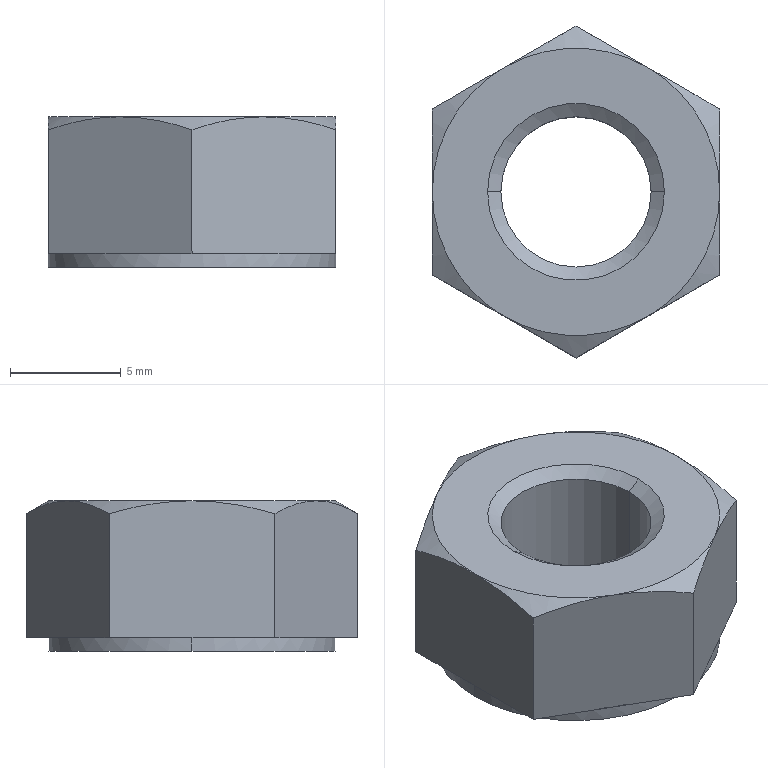Part | STEP file | hex nut style 1 gradeab_iso_ISO - 4032 - M8 - W - N | 1 solid | 30 faces | box 13 x 15.011 x 6.8 mm | volume 731.665 mm3 | plane 14 | cone 10 | cylinder 6 | commonest cylinder face diameters 6.8 x2 8 x2 13 x2
STEP:
#1=CARTESIAN_POINT('',(-4.,0.,-6.8));
#2=VERTEX_POINT('',#1);
#3=CARTESIAN_POINT('',(4.,0.,-6.8));
#4=VERTEX_POINT('',#3);
#5=CARTESIAN_POINT('',(0.,0.,-6.8));
#6=DIRECTION('',(0.,0.,1.));
#7=DIRECTION('',(-1.,0.,0.));
#8=AXIS2_PLACEMENT_3D('',#5,#6,#7);
#9=CIRCLE('',#8,4.);
#10=EDGE_CURVE('',#2,#4,#9,.T.);
#11=ORIENTED_EDGE('',*,*,#10,.F.);
#12=CARTESIAN_POINT('',(-4.,0.,-6.775));
#13=VERTEX_POINT('',#12);
#14=CARTESIAN_POINT('',(-4.,0.,-25.038));
#15=DIRECTION('',(0.,0.,1.));
#16=VECTOR('',#15,1000.);
#17=LINE('',#14,#16);
#18=EDGE_CURVE('',#2,#13,#17,.T.);
#19=ORIENTED_EDGE('',*,*,#18,.T.);
#20=CARTESIAN_POINT('',(4.,0.,-6.775));
#21=VERTEX_POINT('',#20);
#22=CARTESIAN_POINT('',(0.,0.,-6.775));
#23=DIRECTION('',(0.,0.,1.));
#24=DIRECTION('',(1.,0.,0.));
#25=AXIS2_PLACEMENT_3D('',#22,#23,#24);
#26=CIRCLE('',#25,4.);
#27=EDGE_CURVE('',#13,#21,#26,.T.);
#28=ORIENTED_EDGE('',*,*,#27,.T.);
#29=CARTESIAN_POINT('',(4.,0.,-25.038));
#30=DIRECTION('',(0.,0.,1.));
#31=VECTOR('',#30,1000.);
#32=LINE('',#29,#31);
#33=EDGE_CURVE('',#4,#21,#32,.T.);
#34=ORIENTED_EDGE('',*,*,#33,.F.);
#35=EDGE_LOOP('',(#11,#19,#28,#34));
#36=FACE_OUTER_BOUND('',#35,.T.);
#37=CARTESIAN_POINT('',(0.,0.,-25.038));
#38=DIRECTION('',(0.,0.,1.));
#39=DIRECTION('',(1.,0.,0.));
#40=AXIS2_PLACEMENT_3D('',#37,#38,#39);
#41=CYLINDRICAL_SURFACE('',#40,4.);
#42=ADVANCED_FACE('',(#36),#41,.F.);
#43=CARTESIAN_POINT('',(-3.4,0.,-6.354));
#44=VERTEX_POINT('',#43);
#45=CARTESIAN_POINT('',(3.4,0.,-6.354));
#46=VERTEX_POINT('',#45);
#47=CARTESIAN_POINT('',(0.,0.,-6.354));
#48=DIRECTION('',(0.,0.,1.));
#49=DIRECTION('',(-1.,0.,0.));
#50=AXIS2_PLACEMENT_3D('',#47,#48,#49);
#51=CIRCLE('',#50,3.4);
#52=EDGE_CURVE('',#44,#46,#51,.T.);
#53=ORIENTED_EDGE('',*,*,#52,.T.);
#54=CARTESIAN_POINT('',(4.,0.,-6.775));
#55=DIRECTION('',(0.8192,0.,-0.5736));
#56=VECTOR('',#55,1000.);
#57=LINE('',#54,#56);
#58=EDGE_CURVE('',#46,#21,#57,.T.);
#59=ORIENTED_EDGE('',*,*,#58,.T.);
#60=ORIENTED_EDGE('',*,*,#27,.F.);
#61=CARTESIAN_POINT('',(-4.,0.,-6.775));
#62=DIRECTION('',(-0.8192,0.,-0.5736));
#63=VECTOR('',#62,1000.);
#64=LINE('',#61,#63);
#65=EDGE_CURVE('',#44,#13,#64,.T.);
#66=ORIENTED_EDGE('',*,*,#65,.F.);
#67=EDGE_LOOP('',(#53,#59,#60,#66));
#68=FACE_OUTER_BOUND('',#67,.T.);
#69=CARTESIAN_POINT('',(0.,0.,-6.775));
#70=DIRECTION('',(0.,0.,-1.));
#71=DIRECTION('',(-1.,0.,0.));
#72=AXIS2_PLACEMENT_3D('',#69,#70,#71);
#73=CONICAL_SURFACE('',#72,4.,0.9599);
#74=ADVANCED_FACE('',(#68),#73,.F.);
#75=CARTESIAN_POINT('',(3.4,0.,-0.4201));
#76=VERTEX_POINT('',#75);
#77=CARTESIAN_POINT('',(-3.4,0.,-0.4201));
#78=VERTEX_POINT('',#77);
#79=CARTESIAN_POINT('',(0.,0.,-0.4201));
#80=DIRECTION('',(0.,0.,-1.));
#81=DIRECTION('',(1.,0.,0.));
#82=AXIS2_PLACEMENT_3D('',#79,#80,#81);
#83=CIRCLE('',#82,3.4);
#84=EDGE_CURVE('',#76,#78,#83,.T.);
#85=ORIENTED_EDGE('',*,*,#84,.T.);
#86=CARTESIAN_POINT('',(-4.,0.,0.));
#87=VERTEX_POINT('',#86);
#88=CARTESIAN_POINT('',(-3.34,0.,-0.4621));
#89=DIRECTION('',(-0.8192,0.,0.5736));
#90=VECTOR('',#89,1000.);
#91=LINE('',#88,#90);
#92=EDGE_CURVE('',#78,#87,#91,.T.);
#93=ORIENTED_EDGE('',*,*,#92,.T.);
#94=CARTESIAN_POINT('',(4.,0.,0.));
#95=VERTEX_POINT('',#94);
#96=CARTESIAN_POINT('',(0.,0.,0.));
#97=DIRECTION('',(0.,0.,1.));
#98=DIRECTION('',(1.,0.,0.));
#99=AXIS2_PLACEMENT_3D('',#96,#97,#98);
#100=CIRCLE('',#99,4.);
#101=EDGE_CURVE('',#87,#95,#100,.T.);
#102=ORIENTED_EDGE('',*,*,#101,.T.);
#103=CARTESIAN_POINT('',(3.34,0.,-0.4621));
#104=DIRECTION('',(0.8192,0.,0.5736));
#105=VECTOR('',#104,1000.);
#106=LINE('',#103,#105);
#107=EDGE_CURVE('',#76,#95,#106,.T.);
#108=ORIENTED_EDGE('',*,*,#107,.F.);
#109=EDGE_LOOP('',(#85,#93,#102,#108));
#110=FACE_OUTER_BOUND('',#109,.T.);
#111=CARTESIAN_POINT('',(0.,0.,-0.4621));
#112=DIRECTION('',(0.,0.,1.));
#113=DIRECTION('',(1.,0.,0.));
#114=AXIS2_PLACEMENT_3D('',#111,#112,#113);
#115=CONICAL_SURFACE('',#114,3.34,0.9599);
#116=ADVANCED_FACE('',(#110),#115,.F.);
#117=CARTESIAN_POINT('',(6.5,0.,-6.8));
#118=VERTEX_POINT('',#117);
#119=CARTESIAN_POINT('',(-6.5,0.,-6.8));
#120=VERTEX_POINT('',#119);
#121=CARTESIAN_POINT('',(0.,0.,-6.8));
#122=DIRECTION('',(0.,0.,1.));
#123=DIRECTION('',(-1.,0.,0.));
#124=AXIS2_PLACEMENT_3D('',#121,#122,#123);
#125=CIRCLE('',#124,6.5);
#126=EDGE_CURVE('',#118,#120,#125,.T.);
#127=ORIENTED_EDGE('',*,*,#126,.T.);
#128=CARTESIAN_POINT('',(-6.5,0.,-6.2));
#129=VERTEX_POINT('',#128);
#130=CARTESIAN_POINT('',(-6.5,0.,0.));
#131=DIRECTION('',(0.,0.,1.));
#132=VECTOR('',#131,1000.);
#133=LINE('',#130,#132);
#134=EDGE_CURVE('',#120,#129,#133,.T.);
#135=ORIENTED_EDGE('',*,*,#134,.T.);
#136=CARTESIAN_POINT('',(-3.25,5.629,-6.2));
#137=VERTEX_POINT('',#136);
#138=CARTESIAN_POINT('',(0.,0.,-6.2));
#139=DIRECTION('',(0.,0.,1.));
#140=DIRECTION('',(1.,0.,0.));
#141=AXIS2_PLACEMENT_3D('',#138,#139,#140);
#142=CIRCLE('',#141,6.5);
#143=EDGE_CURVE('',#137,#129,#142,.T.);
#144=ORIENTED_EDGE('',*,*,#143,.F.);
#145=CARTESIAN_POINT('',(3.25,5.629,-6.2));
#146=VERTEX_POINT('',#145);
#147=CARTESIAN_POINT('',(0.,0.,-6.2));
#148=DIRECTION('',(0.,0.,1.));
#149=DIRECTION('',(1.,0.,0.));
#150=AXIS2_PLACEMENT_3D('',#147,#148,#149);
#151=CIRCLE('',#150,6.5);
#152=EDGE_CURVE('',#146,#137,#151,.T.);
#153=ORIENTED_EDGE('',*,*,#152,.F.);
#154=CARTESIAN_POINT('',(6.5,0.,-6.2));
#155=VERTEX_POINT('',#154);
#156=CARTESIAN_POINT('',(0.,0.,-6.2));
#157=DIRECTION('',(0.,0.,1.));
#158=DIRECTION('',(1.,0.,0.));
#159=AXIS2_PLACEMENT_3D('',#156,#157,#158);
#160=CIRCLE('',#159,6.5);
#161=EDGE_CURVE('',#155,#146,#160,.T.);
#162=ORIENTED_EDGE('',*,*,#161,.F.);
#163=CARTESIAN_POINT('',(6.5,0.,0.));
#164=DIRECTION('',(0.,0.,1.));
#165=VECTOR('',#164,1000.);
#166=LINE('',#163,#165);
#167=EDGE_CURVE('',#118,#155,#166,.T.);
#168=ORIENTED_EDGE('',*,*,#167,.F.);
#169=EDGE_LOOP('',(#127,#135,#144,#153,#162,#168));
#170=FACE_OUTER_BOUND('',#169,.T.);
#171=CARTESIAN_POINT('',(0.,0.,0.));
#172=DIRECTION('',(0.,0.,1.));
#173=DIRECTION('',(1.,0.,0.));
#174=AXIS2_PLACEMENT_3D('',#171,#172,#173);
#175=CYLINDRICAL_SURFACE('',#174,6.5);
#176=ADVANCED_FACE('',(#170),#175,.T.);
#177=ORIENTED_EDGE('',*,*,#52,.F.);
#178=CARTESIAN_POINT('',(-3.4,0.,-6.8));
#179=DIRECTION('',(0.,0.,1.));
#180=VECTOR('',#179,1000.);
#181=LINE('',#178,#180);
#182=EDGE_CURVE('',#44,#78,#181,.T.);
#183=ORIENTED_EDGE('',*,*,#182,.T.);
#184=ORIENTED_EDGE('',*,*,#84,.F.);
#185=CARTESIAN_POINT('',(3.4,0.,-6.8));
#186=DIRECTION('',(0.,0.,1.));
#187=VECTOR('',#186,1000.);
#188=LINE('',#185,#187);
#189=EDGE_CURVE('',#46,#76,#188,.T.);
#190=ORIENTED_EDGE('',*,*,#189,.F.);
#191=EDGE_LOOP('',(#177,#183,#184,#190));
#192=FACE_OUTER_BOUND('',#191,.T.);
#193=CARTESIAN_POINT('',(0.,0.,-6.8));
#194=DIRECTION('',(0.,0.,1.));
#195=DIRECTION('',(1.,0.,0.));
#196=AXIS2_PLACEMENT_3D('',#193,#194,#195);
#197=CYLINDRICAL_SURFACE('',#196,3.4);
#198=ADVANCED_FACE('',(#192),#197,.F.);
#199=ORIENTED_EDGE('',*,*,#182,.F.);
#200=CARTESIAN_POINT('',(0.,0.,-6.354));
#201=DIRECTION('',(0.,0.,1.));
#202=DIRECTION('',(-1.,0.,0.));
#203=AXIS2_PLACEMENT_3D('',#200,#201,#202);
#204=CIRCLE('',#203,3.4);
#205=EDGE_CURVE('',#46,#44,#204,.T.);
#206=ORIENTED_EDGE('',*,*,#205,.F.);
#207=ORIENTED_EDGE('',*,*,#189,.T.);
#208=CARTESIAN_POINT('',(0.,0.,-0.4201));
#209=DIRECTION('',(0.,0.,-1.));
#210=DIRECTION('',(1.,0.,0.));
#211=AXIS2_PLACEMENT_3D('',#208,#209,#210);
#212=CIRCLE('',#211,3.4);
#213=EDGE_CURVE('',#78,#76,#212,.T.);
#214=ORIENTED_EDGE('',*,*,#213,.F.);
#215=EDGE_LOOP('',(#199,#206,#207,#214));
#216=FACE_OUTER_BOUND('',#215,.T.);
#217=CARTESIAN_POINT('',(0.,0.,-6.8));
#218=DIRECTION('',(0.,0.,1.));
#219=DIRECTION('',(1.,0.,0.));
#220=AXIS2_PLACEMENT_3D('',#217,#218,#219);
#221=CYLINDRICAL_SURFACE('',#220,3.4);
#222=ADVANCED_FACE('',(#216),#221,.F.);
#223=CARTESIAN_POINT('',(-6.5,3.753,-6.2));
#224=VERTEX_POINT('',#223);
#225=CARTESIAN_POINT('',(-6.5,3.753,-0.5806));
#226=VERTEX_POINT('',#225);
#227=CARTESIAN_POINT('',(-6.5,3.753,-6.8));
#228=DIRECTION('',(0.,0.,1.));
#229=VECTOR('',#228,1000.);
#230=LINE('',#227,#229);
#231=EDGE_CURVE('',#224,#226,#230,.T.);
#232=ORIENTED_EDGE('',*,*,#231,.T.);
#233=CARTESIAN_POINT('',(-3.25,5.629,0.));
#234=VERTEX_POINT('',#233);
#235=CARTESIAN_POINT('',(-6.5,3.753,-0.5806));
#236=CARTESIAN_POINT('',(-5.968,4.06,-0.4033));
#237=CARTESIAN_POINT('',(-5.433,4.369,-0.2573));
#238=CARTESIAN_POINT('',(-4.351,4.994,-0.05533));
#239=CARTESIAN_POINT('',(-3.804,5.309,0.));
#240=CARTESIAN_POINT('',(-3.25,5.629,0.));
#241=B_SPLINE_CURVE_WITH_KNOTS('',3,(#235,#236,#237,#238,#239,#240),.UNSPECIFIED.,.F.,.F.,(4,2,4),(0.000000238,0.001899,0.003797),.UNSPECIFIED.);
#242=EDGE_CURVE('',#226,#234,#241,.T.);
#243=ORIENTED_EDGE('',*,*,#242,.T.);
#244=CARTESIAN_POINT('',(0.,7.506,-0.5806));
#245=VERTEX_POINT('',#244);
#246=CARTESIAN_POINT('',(-3.25,5.629,0.));
#247=CARTESIAN_POINT('',(-2.974,5.788,0.));
#248=CARTESIAN_POINT('',(-2.697,5.948,-0.01372));
#249=CARTESIAN_POINT('',(-2.149,6.265,-0.06683));
#250=CARTESIAN_POINT('',(-1.877,6.422,-0.1062));
#251=CARTESIAN_POINT('',(-1.065,6.891,-0.2578));
#252=CARTESIAN_POINT('',(-0.5303,7.199,-0.4038));
#253=CARTESIAN_POINT('',(0.,7.506,-0.5806));
#254=B_SPLINE_CURVE_WITH_KNOTS('',3,(#246,#247,#248,#249,#250,#251,#252,#253),.UNSPECIFIED.,.F.,.F.,(4,2,2,4),(0.003797,0.004743,0.005689,0.00758),.UNSPECIFIED.);
#255=EDGE_CURVE('',#234,#245,#254,.T.);
#256=ORIENTED_EDGE('',*,*,#255,.T.);
#257=CARTESIAN_POINT('',(0.,7.506,-6.2));
#258=VERTEX_POINT('',#257);
#259=CARTESIAN_POINT('',(0.,7.506,-6.8));
#260=DIRECTION('',(0.,0.,1.));
#261=VECTOR('',#260,1000.);
#262=LINE('',#259,#261);
#263=EDGE_CURVE('',#258,#245,#262,.T.);
#264=ORIENTED_EDGE('',*,*,#263,.F.);
#265=CARTESIAN_POINT('',(0.,7.506,-6.2));
#266=DIRECTION('',(-0.866,-0.5,0.));
#267=VECTOR('',#266,1000.);
#268=LINE('',#265,#267);
#269=EDGE_CURVE('',#258,#137,#268,.T.);
#270=ORIENTED_EDGE('',*,*,#269,.T.);
#271=CARTESIAN_POINT('',(0.,7.506,-6.2));
#272=DIRECTION('',(-0.866,-0.5,0.));
#273=VECTOR('',#272,1000.);
#274=LINE('',#271,#273);
#275=EDGE_CURVE('',#137,#224,#274,.T.);
#276=ORIENTED_EDGE('',*,*,#275,.T.);
#277=EDGE_LOOP('',(#232,#243,#256,#264,#270,#276));
#278=FACE_OUTER_BOUND('',#277,.T.);
#279=CARTESIAN_POINT('',(0.,7.506,-6.8));
#280=DIRECTION('',(-0.5,0.866,0.));
#281=DIRECTION('',(-0.866,-0.5,0.));
#282=AXIS2_PLACEMENT_3D('',#279,#280,#281);
#283=PLANE('',#282);
#284=ADVANCED_FACE('',(#278),#283,.T.);
#285=ORIENTED_EDGE('',*,*,#263,.T.);
#286=CARTESIAN_POINT('',(3.25,5.629,0.));
#287=VERTEX_POINT('',#286);
#288=CARTESIAN_POINT('',(0.,7.506,-0.5806));
#289=CARTESIAN_POINT('',(0.5317,7.199,-0.4033));
#290=CARTESIAN_POINT('',(1.067,6.889,-0.2573));
#291=CARTESIAN_POINT('',(2.149,6.265,-0.05533));
#292=CARTESIAN_POINT('',(2.696,5.949,0.));
#293=CARTESIAN_POINT('',(3.25,5.629,0.));
#294=B_SPLINE_CURVE_WITH_KNOTS('',3,(#288,#289,#290,#291,#292,#293),.UNSPECIFIED.,.F.,.F.,(4,2,4),(0.000000238,0.001899,0.003797),.UNSPECIFIED.);
#295=EDGE_CURVE('',#245,#287,#294,.T.);
#296=ORIENTED_EDGE('',*,*,#295,.T.);
#297=CARTESIAN_POINT('',(6.5,3.753,-0.5806));
#298=VERTEX_POINT('',#297);
#299=CARTESIAN_POINT('',(3.25,5.629,0.));
#300=CARTESIAN_POINT('',(3.526,5.47,0.));
#301=CARTESIAN_POINT('',(3.803,5.31,-0.01372));
#302=CARTESIAN_POINT('',(4.351,4.994,-0.06683));
#303=CARTESIAN_POINT('',(4.623,4.836,-0.1062));
#304=CARTESIAN_POINT('',(5.435,4.368,-0.2578));
#305=CARTESIAN_POINT('',(5.97,4.059,-0.4038));
#306=CARTESIAN_POINT('',(6.5,3.753,-0.5806));
#307=B_SPLINE_CURVE_WITH_KNOTS('',3,(#299,#300,#301,#302,#303,#304,#305,#306),.UNSPECIFIED.,.F.,.F.,(4,2,2,4),(0.003797,0.004743,0.005689,0.00758),.UNSPECIFIED.);
#308=EDGE_CURVE('',#287,#298,#307,.T.);
#309=ORIENTED_EDGE('',*,*,#308,.T.);
#310=CARTESIAN_POINT('',(6.5,3.753,-6.2));
#311=VERTEX_POINT('',#310);
#312=CARTESIAN_POINT('',(6.5,3.753,-6.8));
#313=DIRECTION('',(0.,0.,1.));
#314=VECTOR('',#313,1000.);
#315=LINE('',#312,#314);
#316=EDGE_CURVE('',#311,#298,#315,.T.);
#317=ORIENTED_EDGE('',*,*,#316,.F.);
#318=CARTESIAN_POINT('',(6.5,3.753,-6.2));
#319=DIRECTION('',(-0.866,0.5,0.));
#320=VECTOR('',#319,1000.);
#321=LINE('',#318,#320);
#322=EDGE_CURVE('',#311,#146,#321,.T.);
#323=ORIENTED_EDGE('',*,*,#322,.T.);
#324=CARTESIAN_POINT('',(6.5,3.753,-6.2));
#325=DIRECTION('',(-0.866,0.5,0.));
#326=VECTOR('',#325,1000.);
#327=LINE('',#324,#326);
#328=EDGE_CURVE('',#146,#258,#327,.T.);
#329=ORIENTED_EDGE('',*,*,#328,.T.);
#330=EDGE_LOOP('',(#285,#296,#309,#317,#323,#329));
#331=FACE_OUTER_BOUND('',#330,.T.);
#332=CARTESIAN_POINT('',(6.5,3.753,-6.8));
#333=DIRECTION('',(0.5,0.866,0.));
#334=DIRECTION('',(-0.866,0.5,0.));
#335=AXIS2_PLACEMENT_3D('',#332,#333,#334);
#336=PLANE('',#335);
#337=ADVANCED_FACE('',(#331),#336,.T.);
#338=CARTESIAN_POINT('',(6.5,-3.753,-0.5806));
#339=VERTEX_POINT('',#338);
#340=CARTESIAN_POINT('',(6.5,0.,0.));
#341=VERTEX_POINT('',#340);
#342=CARTESIAN_POINT('',(6.5,-3.753,-0.5806));
#343=CARTESIAN_POINT('',(6.5,-3.142,-0.4044));
#344=CARTESIAN_POINT('',(6.5,-2.517,-0.2566));
#345=CARTESIAN_POINT('',(6.5,-1.264,-0.05451));
#346=CARTESIAN_POINT('',(6.5,-0.6342,0.));
#347=CARTESIAN_POINT('',(6.5,0.,0.));
#348=B_SPLINE_CURVE_WITH_KNOTS('',3,(#342,#343,#344,#345,#346,#347),.UNSPECIFIED.,.F.,.F.,(4,2,4),(0.006695,0.008594,0.01049),.UNSPECIFIED.);
#349=EDGE_CURVE('',#339,#341,#348,.T.);
#350=ORIENTED_EDGE('',*,*,#349,.F.);
#351=CARTESIAN_POINT('',(6.5,-3.753,-6.2));
#352=VERTEX_POINT('',#351);
#353=CARTESIAN_POINT('',(6.5,-3.753,-6.8));
#354=DIRECTION('',(0.,0.,1.));
#355=VECTOR('',#354,1000.);
#356=LINE('',#353,#355);
#357=EDGE_CURVE('',#352,#339,#356,.T.);
#358=ORIENTED_EDGE('',*,*,#357,.F.);
#359=CARTESIAN_POINT('',(6.5,3.753,-6.2));
#360=DIRECTION('',(0.,-1.,0.));
#361=VECTOR('',#360,1000.);
#362=LINE('',#359,#361);
#363=EDGE_CURVE('',#155,#352,#362,.T.);
#364=ORIENTED_EDGE('',*,*,#363,.F.);
#365=CARTESIAN_POINT('',(6.5,3.753,-6.2));
#366=DIRECTION('',(0.,-1.,0.));
#367=VECTOR('',#366,1000.);
#368=LINE('',#365,#367);
#369=EDGE_CURVE('',#311,#155,#368,.T.);
#370=ORIENTED_EDGE('',*,*,#369,.F.);
#371=ORIENTED_EDGE('',*,*,#316,.T.);
#372=CARTESIAN_POINT('',(6.5,0.,0.));
#373=CARTESIAN_POINT('',(6.5,0.6345,0.));
#374=CARTESIAN_POINT('',(6.5,1.278,-0.05602));
#375=CARTESIAN_POINT('',(6.5,2.531,-0.2595));
#376=CARTESIAN_POINT('',(6.5,3.146,-0.4054));
#377=CARTESIAN_POINT('',(6.5,3.753,-0.5806));
#378=B_SPLINE_CURVE_WITH_KNOTS('',3,(#372,#373,#374,#375,#376,#377),.UNSPECIFIED.,.F.,.F.,(4,2,4),(0.01049,0.01239,0.01429),.UNSPECIFIED.);
#379=EDGE_CURVE('',#341,#298,#378,.T.);
#380=ORIENTED_EDGE('',*,*,#379,.F.);
#381=EDGE_LOOP('',(#350,#358,#364,#370,#371,#380));
#382=FACE_OUTER_BOUND('',#381,.T.);
#383=CARTESIAN_POINT('',(6.5,3.753,-6.8));
#384=DIRECTION('',(-1.,0.,0.));
#385=DIRECTION('',(0.,0.,1.));
#386=AXIS2_PLACEMENT_3D('',#383,#384,#385);
#387=PLANE('',#386);
#388=ADVANCED_FACE('',(#382),#387,.F.);
#389=ORIENTED_EDGE('',*,*,#357,.T.);
#390=CARTESIAN_POINT('',(3.25,-5.629,0.));
#391=VERTEX_POINT('',#390);
#392=CARTESIAN_POINT('',(6.5,-3.753,-0.5806));
#393=CARTESIAN_POINT('',(5.968,-4.06,-0.4033));
#394=CARTESIAN_POINT('',(5.433,-4.369,-0.2573));
#395=CARTESIAN_POINT('',(4.351,-4.994,-0.05533));
#396=CARTESIAN_POINT('',(3.804,-5.309,0.));
#397=CARTESIAN_POINT('',(3.25,-5.629,0.));
#398=B_SPLINE_CURVE_WITH_KNOTS('',3,(#392,#393,#394,#395,#396,#397),.UNSPECIFIED.,.F.,.F.,(4,2,4),(0.000000238,0.001899,0.003797),.UNSPECIFIED.);
#399=EDGE_CURVE('',#339,#391,#398,.T.);
#400=ORIENTED_EDGE('',*,*,#399,.T.);
#401=CARTESIAN_POINT('',(0.,-7.506,-0.5806));
#402=VERTEX_POINT('',#401);
#403=CARTESIAN_POINT('',(3.25,-5.629,0.));
#404=CARTESIAN_POINT('',(2.974,-5.788,0.));
#405=CARTESIAN_POINT('',(2.697,-5.948,-0.01372));
#406=CARTESIAN_POINT('',(2.149,-6.265,-0.06683));
#407=CARTESIAN_POINT('',(1.877,-6.422,-0.1062));
#408=CARTESIAN_POINT('',(1.065,-6.891,-0.2578));
#409=CARTESIAN_POINT('',(0.5303,-7.199,-0.4038));
#410=CARTESIAN_POINT('',(0.,-7.506,-0.5806));
#411=B_SPLINE_CURVE_WITH_KNOTS('',3,(#403,#404,#405,#406,#407,#408,#409,#410),.UNSPECIFIED.,.F.,.F.,(4,2,2,4),(0.003797,0.004743,0.005689,0.00758),.UNSPECIFIED.);
#412=EDGE_CURVE('',#391,#402,#411,.T.);
#413=ORIENTED_EDGE('',*,*,#412,.T.);
#414=CARTESIAN_POINT('',(0.,-7.506,-6.2));
#415=VERTEX_POINT('',#414);
#416=CARTESIAN_POINT('',(0.,-7.506,-6.8));
#417=DIRECTION('',(0.,0.,1.));
#418=VECTOR('',#417,1000.);
#419=LINE('',#416,#418);
#420=EDGE_CURVE('',#415,#402,#419,.T.);
#421=ORIENTED_EDGE('',*,*,#420,.F.);
#422=CARTESIAN_POINT('',(3.25,-5.629,-6.2));
#423=VERTEX_POINT('',#422);
#424=CARTESIAN_POINT('',(0.,-7.506,-6.2));
#425=DIRECTION('',(0.866,0.5,0.));
#426=VECTOR('',#425,1000.);
#427=LINE('',#424,#426);
#428=EDGE_CURVE('',#415,#423,#427,.T.);
#429=ORIENTED_EDGE('',*,*,#428,.T.);
#430=CARTESIAN_POINT('',(0.,-7.506,-6.2));
#431=DIRECTION('',(0.866,0.5,0.));
#432=VECTOR('',#431,1000.);
#433=LINE('',#430,#432);
#434=EDGE_CURVE('',#423,#352,#433,.T.);
#435=ORIENTED_EDGE('',*,*,#434,.T.);
#436=EDGE_LOOP('',(#389,#400,#413,#421,#429,#435));
#437=FACE_OUTER_BOUND('',#436,.T.);
#438=CARTESIAN_POINT('',(0.,-7.506,-6.8));
#439=DIRECTION('',(0.5,-0.866,0.));
#440=DIRECTION('',(0.866,0.5,0.));
#441=AXIS2_PLACEMENT_3D('',#438,#439,#440);
#442=PLANE('',#441);
#443=ADVANCED_FACE('',(#437),#442,.T.);
#444=ORIENTED_EDGE('',*,*,#420,.T.);
#445=CARTESIAN_POINT('',(-3.25,-5.629,0.));
#446=VERTEX_POINT('',#445);
#447=CARTESIAN_POINT('',(0.,-7.506,-0.5806));
#448=CARTESIAN_POINT('',(-0.5317,-7.199,-0.4033));
#449=CARTESIAN_POINT('',(-1.067,-6.889,-0.2573));
#450=CARTESIAN_POINT('',(-2.149,-6.265,-0.05533));
#451=CARTESIAN_POINT('',(-2.696,-5.949,0.));
#452=CARTESIAN_POINT('',(-3.25,-5.629,0.));
#453=B_SPLINE_CURVE_WITH_KNOTS('',3,(#447,#448,#449,#450,#451,#452),.UNSPECIFIED.,.F.,.F.,(4,2,4),(0.000000238,0.001899,0.003797),.UNSPECIFIED.);
#454=EDGE_CURVE('',#402,#446,#453,.T.);
#455=ORIENTED_EDGE('',*,*,#454,.T.);
#456=CARTESIAN_POINT('',(-6.5,-3.753,-0.5806));
#457=VERTEX_POINT('',#456);
#458=CARTESIAN_POINT('',(-3.25,-5.629,0.));
#459=CARTESIAN_POINT('',(-3.526,-5.47,0.));
#460=CARTESIAN_POINT('',(-3.803,-5.31,-0.01372));
#461=CARTESIAN_POINT('',(-4.351,-4.994,-0.06683));
#462=CARTESIAN_POINT('',(-4.623,-4.836,-0.1062));
#463=CARTESIAN_POINT('',(-5.435,-4.368,-0.2578));
#464=CARTESIAN_POINT('',(-5.97,-4.059,-0.4038));
#465=CARTESIAN_POINT('',(-6.5,-3.753,-0.5806));
#466=B_SPLINE_CURVE_WITH_KNOTS('',3,(#458,#459,#460,#461,#462,#463,#464,#465),.UNSPECIFIED.,.F.,.F.,(4,2,2,4),(0.003797,0.004743,0.005689,0.00758),.UNSPECIFIED.);
#467=EDGE_CURVE('',#446,#457,#466,.T.);
#468=ORIENTED_EDGE('',*,*,#467,.T.);
#469=CARTESIAN_POINT('',(-6.5,-3.753,-6.2));
#470=VERTEX_POINT('',#469);
#471=CARTESIAN_POINT('',(-6.5,-3.753,-6.8));
#472=DIRECTION('',(0.,0.,1.));
#473=VECTOR('',#472,1000.);
#474=LINE('',#471,#473);
#475=EDGE_CURVE('',#470,#457,#474,.T.);
#476=ORIENTED_EDGE('',*,*,#475,.F.);
#477=CARTESIAN_POINT('',(-3.25,-5.629,-6.2));
#478=VERTEX_POINT('',#477);
#479=CARTESIAN_POINT('',(-6.5,-3.753,-6.2));
#480=DIRECTION('',(0.866,-0.5,0.));
#481=VECTOR('',#480,1000.);
#482=LINE('',#479,#481);
#483=EDGE_CURVE('',#470,#478,#482,.T.);
#484=ORIENTED_EDGE('',*,*,#483,.T.);
#485=CARTESIAN_POINT('',(-6.5,-3.753,-6.2));
#486=DIRECTION('',(0.866,-0.5,0.));
#487=VECTOR('',#486,1000.);
#488=LINE('',#485,#487);
#489=EDGE_CURVE('',#478,#415,#488,.T.);
#490=ORIENTED_EDGE('',*,*,#489,.T.);
#491=EDGE_LOOP('',(#444,#455,#468,#476,#484,#490));
#492=FACE_OUTER_BOUND('',#491,.T.);
#493=CARTESIAN_POINT('',(-6.5,-3.753,-6.8));
#494=DIRECTION('',(-0.5,-0.866,0.));
#495=DIRECTION('',(0.866,-0.5,0.));
#496=AXIS2_PLACEMENT_3D('',#493,#494,#495);
#497=PLANE('',#496);
#498=ADVANCED_FACE('',(#492),#497,.T.);
#499=ORIENTED_EDGE('',*,*,#475,.T.);
#500=CARTESIAN_POINT('',(-6.5,0.,0.));
#501=VERTEX_POINT('',#500);
#502=CARTESIAN_POINT('',(-6.5,-3.753,-0.5806));
#503=CARTESIAN_POINT('',(-6.5,-3.142,-0.4044));
#504=CARTESIAN_POINT('',(-6.5,-2.517,-0.2566));
#505=CARTESIAN_POINT('',(-6.5,-1.264,-0.05451));
#506=CARTESIAN_POINT('',(-6.5,-0.6342,0.));
#507=CARTESIAN_POINT('',(-6.5,0.,0.));
#508=B_SPLINE_CURVE_WITH_KNOTS('',3,(#502,#503,#504,#505,#506,#507),.UNSPECIFIED.,.F.,.F.,(4,2,4),(0.006695,0.008594,0.01049),.UNSPECIFIED.);
#509=EDGE_CURVE('',#457,#501,#508,.T.);
#510=ORIENTED_EDGE('',*,*,#509,.T.);
#511=CARTESIAN_POINT('',(-6.5,0.,0.));
#512=CARTESIAN_POINT('',(-6.5,0.6345,0.));
#513=CARTESIAN_POINT('',(-6.5,1.278,-0.05602));
#514=CARTESIAN_POINT('',(-6.5,2.531,-0.2595));
#515=CARTESIAN_POINT('',(-6.5,3.146,-0.4054));
#516=CARTESIAN_POINT('',(-6.5,3.753,-0.5806));
#517=B_SPLINE_CURVE_WITH_KNOTS('',3,(#511,#512,#513,#514,#515,#516),.UNSPECIFIED.,.F.,.F.,(4,2,4),(0.01049,0.01239,0.01429),.UNSPECIFIED.);
#518=EDGE_CURVE('',#501,#226,#517,.T.);
#519=ORIENTED_EDGE('',*,*,#518,.T.);
#520=ORIENTED_EDGE('',*,*,#231,.F.);
#521=CARTESIAN_POINT('',(-6.5,3.753,-6.2));
#522=DIRECTION('',(0.,-1.,0.));
#523=VECTOR('',#522,1000.);
#524=LINE('',#521,#523);
#525=EDGE_CURVE('',#224,#129,#524,.T.);
#526=ORIENTED_EDGE('',*,*,#525,.T.);
#527=CARTESIAN_POINT('',(-6.5,3.753,-6.2));
#528=DIRECTION('',(0.,-1.,0.));
#529=VECTOR('',#528,1000.);
#530=LINE('',#527,#529);
#531=EDGE_CURVE('',#129,#470,#530,.T.);
#532=ORIENTED_EDGE('',*,*,#531,.T.);
#533=EDGE_LOOP('',(#499,#510,#519,#520,#526,#532));
#534=FACE_OUTER_BOUND('',#533,.T.);
#535=CARTESIAN_POINT('',(-6.5,3.753,-6.8));
#536=DIRECTION('',(-1.,0.,0.));
#537=DIRECTION('',(0.,0.,1.));
#538=AXIS2_PLACEMENT_3D('',#535,#536,#537);
#539=PLANE('',#538);
#540=ADVANCED_FACE('',(#534),#539,.T.);
#541=CARTESIAN_POINT('',(0.,0.,0.));
#542=DIRECTION('',(0.,0.,1.));
#543=DIRECTION('',(1.,0.,0.));
#544=AXIS2_PLACEMENT_3D('',#541,#542,#543);
#545=CIRCLE('',#544,4.);
#546=EDGE_CURVE('',#95,#87,#545,.T.);
#547=ORIENTED_EDGE('',*,*,#546,.F.);
#548=ORIENTED_EDGE('',*,*,#101,.F.);
#549=EDGE_LOOP('',(#547,#548));
#550=FACE_BOUND('',#549,.T.);
#551=CARTESIAN_POINT('',(0.,0.,0.));
#552=DIRECTION('',(0.,0.,1.));
#553=DIRECTION('',(-1.,0.,0.));
#554=AXIS2_PLACEMENT_3D('',#551,#552,#553);
#555=CIRCLE('',#554,6.5);
#556=EDGE_CURVE('',#234,#501,#555,.T.);
#557=ORIENTED_EDGE('',*,*,#556,.T.);
#558=CARTESIAN_POINT('',(0.,0.,0.));
#559=DIRECTION('',(0.,0.,1.));
#560=DIRECTION('',(-1.,0.,0.));
#561=AXIS2_PLACEMENT_3D('',#558,#559,#560);
#562=CIRCLE('',#561,6.5);
#563=EDGE_CURVE('',#501,#446,#562,.T.);
#564=ORIENTED_EDGE('',*,*,#563,.T.);
#565=CARTESIAN_POINT('',(0.,0.,0.));
#566=DIRECTION('',(0.,0.,1.));
#567=DIRECTION('',(-1.,0.,0.));
#568=AXIS2_PLACEMENT_3D('',#565,#566,#567);
#569=CIRCLE('',#568,6.5);
#570=EDGE_CURVE('',#446,#391,#569,.T.);
#571=ORIENTED_EDGE('',*,*,#570,.T.);
#572=CARTESIAN_POINT('',(0.,0.,0.));
#573=DIRECTION('',(0.,0.,1.));
#574=DIRECTION('',(-1.,0.,0.));
#575=AXIS2_PLACEMENT_3D('',#572,#573,#574);
#576=CIRCLE('',#575,6.5);
#577=EDGE_CURVE('',#391,#341,#576,.T.);
#578=ORIENTED_EDGE('',*,*,#577,.T.);
#579=CARTESIAN_POINT('',(0.,0.,0.));
#580=DIRECTION('',(0.,0.,1.));
#581=DIRECTION('',(1.,0.,0.));
#582=AXIS2_PLACEMENT_3D('',#579,#580,#581);
#583=CIRCLE('',#582,6.5);
#584=EDGE_CURVE('',#341,#287,#583,.T.);
#585=ORIENTED_EDGE('',*,*,#584,.T.);
#586=CARTESIAN_POINT('',(0.,0.,0.));
#587=DIRECTION('',(0.,0.,1.));
#588=DIRECTION('',(-1.,0.,0.));
#589=AXIS2_PLACEMENT_3D('',#586,#587,#588);
#590=CIRCLE('',#589,6.5);
#591=EDGE_CURVE('',#287,#234,#590,.T.);
#592=ORIENTED_EDGE('',*,*,#591,.T.);
#593=EDGE_LOOP('',(#557,#564,#571,#578,#585,#592));
#594=FACE_OUTER_BOUND('',#593,.T.);
#595=CARTESIAN_POINT('',(0.,7.506,0.));
#596=DIRECTION('',(0.,0.,-1.));
#597=DIRECTION('',(-1.,0.,0.));
#598=AXIS2_PLACEMENT_3D('',#595,#596,#597);
#599=PLANE('',#598);
#600=ADVANCED_FACE('',(#550,#594),#599,.F.);
#601=CARTESIAN_POINT('',(0.,0.,-6.8));
#602=DIRECTION('',(0.,0.,1.));
#603=DIRECTION('',(-1.,0.,0.));
#604=AXIS2_PLACEMENT_3D('',#601,#602,#603);
#605=CIRCLE('',#604,4.);
#606=EDGE_CURVE('',#4,#2,#605,.T.);
#607=ORIENTED_EDGE('',*,*,#606,.T.);
#608=ORIENTED_EDGE('',*,*,#10,.T.);
#609=EDGE_LOOP('',(#607,#608));
#610=FACE_BOUND('',#609,.T.);
#611=ORIENTED_EDGE('',*,*,#126,.F.);
#612=CARTESIAN_POINT('',(0.,0.,-6.8));
#613=DIRECTION('',(0.,0.,1.));
#614=DIRECTION('',(-1.,0.,0.));
#615=AXIS2_PLACEMENT_3D('',#612,#613,#614);
#616=CIRCLE('',#615,6.5);
#617=EDGE_CURVE('',#120,#118,#616,.T.);
#618=ORIENTED_EDGE('',*,*,#617,.F.);
#619=EDGE_LOOP('',(#611,#618));
#620=FACE_OUTER_BOUND('',#619,.T.);
#621=CARTESIAN_POINT('',(0.,7.506,-6.8));
#622=DIRECTION('',(0.,0.,-1.));
#623=DIRECTION('',(-1.,0.,0.));
#624=AXIS2_PLACEMENT_3D('',#621,#622,#623);
#625=PLANE('',#624);
#626=ADVANCED_FACE('',(#610,#620),#625,.T.);
#627=ORIENTED_EDGE('',*,*,#369,.T.);
#628=ORIENTED_EDGE('',*,*,#161,.T.);
#629=ORIENTED_EDGE('',*,*,#322,.F.);
#630=EDGE_LOOP('',(#627,#628,#629));
#631=FACE_OUTER_BOUND('',#630,.T.);
#632=CARTESIAN_POINT('',(0.,17.506,-6.2));
#633=DIRECTION('',(0.,0.,-1.));
#634=DIRECTION('',(-1.,0.,0.));
#635=AXIS2_PLACEMENT_3D('',#632,#633,#634);
#636=PLANE('',#635);
#637=ADVANCED_FACE('',(#631),#636,.T.);
#638=ORIENTED_EDGE('',*,*,#363,.T.);
#639=ORIENTED_EDGE('',*,*,#434,.F.);
#640=CARTESIAN_POINT('',(0.,0.,-6.2));
#641=DIRECTION('',(0.,0.,1.));
#642=DIRECTION('',(1.,0.,0.));
#643=AXIS2_PLACEMENT_3D('',#640,#641,#642);
#644=CIRCLE('',#643,6.5);
#645=EDGE_CURVE('',#423,#155,#644,.T.);
#646=ORIENTED_EDGE('',*,*,#645,.T.);
#647=EDGE_LOOP('',(#638,#639,#646));
#648=FACE_OUTER_BOUND('',#647,.T.);
#649=CARTESIAN_POINT('',(0.,17.506,-6.2));
#650=DIRECTION('',(0.,0.,-1.));
#651=DIRECTION('',(-1.,0.,0.));
#652=AXIS2_PLACEMENT_3D('',#649,#650,#651);
#653=PLANE('',#652);
#654=ADVANCED_FACE('',(#648),#653,.T.);
#655=ORIENTED_EDGE('',*,*,#152,.T.);
#656=ORIENTED_EDGE('',*,*,#269,.F.);
#657=ORIENTED_EDGE('',*,*,#328,.F.);
#658=EDGE_LOOP('',(#655,#656,#657));
#659=FACE_OUTER_BOUND('',#658,.T.);
#660=CARTESIAN_POINT('',(0.,17.506,-6.2));
#661=DIRECTION('',(0.,0.,-1.));
#662=DIRECTION('',(-1.,0.,0.));
#663=AXIS2_PLACEMENT_3D('',#660,#661,#662);
#664=PLANE('',#663);
#665=ADVANCED_FACE('',(#659),#664,.T.);
#666=ORIENTED_EDGE('',*,*,#489,.F.);
#667=CARTESIAN_POINT('',(0.,0.,-6.2));
#668=DIRECTION('',(0.,0.,1.));
#669=DIRECTION('',(1.,0.,0.));
#670=AXIS2_PLACEMENT_3D('',#667,#668,#669);
#671=CIRCLE('',#670,6.5);
#672=EDGE_CURVE('',#478,#423,#671,.T.);
#673=ORIENTED_EDGE('',*,*,#672,.T.);
#674=ORIENTED_EDGE('',*,*,#428,.F.);
#675=EDGE_LOOP('',(#666,#673,#674));
#676=FACE_OUTER_BOUND('',#675,.T.);
#677=CARTESIAN_POINT('',(0.,17.506,-6.2));
#678=DIRECTION('',(0.,0.,-1.));
#679=DIRECTION('',(-1.,0.,0.));
#680=AXIS2_PLACEMENT_3D('',#677,#678,#679);
#681=PLANE('',#680);
#682=ADVANCED_FACE('',(#676),#681,.T.);
#683=ORIENTED_EDGE('',*,*,#143,.T.);
#684=ORIENTED_EDGE('',*,*,#525,.F.);
#685=ORIENTED_EDGE('',*,*,#275,.F.);
#686=EDGE_LOOP('',(#683,#684,#685));
#687=FACE_OUTER_BOUND('',#686,.T.);
#688=CARTESIAN_POINT('',(0.,17.506,-6.2));
#689=DIRECTION('',(0.,0.,-1.));
#690=DIRECTION('',(-1.,0.,0.));
#691=AXIS2_PLACEMENT_3D('',#688,#689,#690);
#692=PLANE('',#691);
#693=ADVANCED_FACE('',(#687),#692,.T.);
#694=ORIENTED_EDGE('',*,*,#134,.F.);
#695=ORIENTED_EDGE('',*,*,#617,.T.);
#696=ORIENTED_EDGE('',*,*,#167,.T.);
#697=ORIENTED_EDGE('',*,*,#645,.F.);
#698=ORIENTED_EDGE('',*,*,#672,.F.);
#699=CARTESIAN_POINT('',(0.,0.,-6.2));
#700=DIRECTION('',(0.,0.,1.));
#701=DIRECTION('',(1.,0.,0.));
#702=AXIS2_PLACEMENT_3D('',#699,#700,#701);
#703=CIRCLE('',#702,6.5);
#704=EDGE_CURVE('',#129,#478,#703,.T.);
#705=ORIENTED_EDGE('',*,*,#704,.F.);
#706=EDGE_LOOP('',(#694,#695,#696,#697,#698,#705));
#707=FACE_OUTER_BOUND('',#706,.T.);
#708=CARTESIAN_POINT('',(0.,0.,0.));
#709=DIRECTION('',(0.,0.,1.));
#710=DIRECTION('',(1.,0.,0.));
#711=AXIS2_PLACEMENT_3D('',#708,#709,#710);
#712=CYLINDRICAL_SURFACE('',#711,6.5);
#713=ADVANCED_FACE('',(#707),#712,.T.);
#714=ORIENTED_EDGE('',*,*,#531,.F.);
#715=ORIENTED_EDGE('',*,*,#704,.T.);
#716=ORIENTED_EDGE('',*,*,#483,.F.);
#717=EDGE_LOOP('',(#714,#715,#716));
#718=FACE_OUTER_BOUND('',#717,.T.);
#719=CARTESIAN_POINT('',(0.,17.506,-6.2));
#720=DIRECTION('',(0.,0.,-1.));
#721=DIRECTION('',(-1.,0.,0.));
#722=AXIS2_PLACEMENT_3D('',#719,#720,#721);
#723=PLANE('',#722);
#724=ADVANCED_FACE('',(#718),#723,.T.);
#725=ORIENTED_EDGE('',*,*,#518,.F.);
#726=ORIENTED_EDGE('',*,*,#556,.F.);
#727=ORIENTED_EDGE('',*,*,#242,.F.);
#728=EDGE_LOOP('',(#725,#726,#727));
#729=FACE_OUTER_BOUND('',#728,.T.);
#730=CARTESIAN_POINT('',(0.,0.,0.));
#731=DIRECTION('',(0.,0.,-1.));
#732=DIRECTION('',(-1.,0.,0.));
#733=AXIS2_PLACEMENT_3D('',#730,#731,#732);
#734=CONICAL_SURFACE('',#733,6.5,1.047);
#735=ADVANCED_FACE('',(#729),#734,.T.);
#736=ORIENTED_EDGE('',*,*,#591,.F.);
#737=ORIENTED_EDGE('',*,*,#295,.F.);
#738=ORIENTED_EDGE('',*,*,#255,.F.);
#739=EDGE_LOOP('',(#736,#737,#738));
#740=FACE_OUTER_BOUND('',#739,.T.);
#741=CARTESIAN_POINT('',(0.,0.,0.));
#742=DIRECTION('',(0.,0.,-1.));
#743=DIRECTION('',(-1.,0.,0.));
#744=AXIS2_PLACEMENT_3D('',#741,#742,#743);
#745=CONICAL_SURFACE('',#744,6.5,1.047);
#746=ADVANCED_FACE('',(#740),#745,.T.);
#747=ORIENTED_EDGE('',*,*,#584,.F.);
#748=ORIENTED_EDGE('',*,*,#379,.T.);
#749=ORIENTED_EDGE('',*,*,#308,.F.);
#750=EDGE_LOOP('',(#747,#748,#749));
#751=FACE_OUTER_BOUND('',#750,.T.);
#752=CARTESIAN_POINT('',(0.,0.,0.));
#753=DIRECTION('',(0.,0.,-1.));
#754=DIRECTION('',(-1.,0.,0.));
#755=AXIS2_PLACEMENT_3D('',#752,#753,#754);
#756=CONICAL_SURFACE('',#755,6.5,1.047);
#757=ADVANCED_FACE('',(#751),#756,.T.);
#758=ORIENTED_EDGE('',*,*,#349,.T.);
#759=ORIENTED_EDGE('',*,*,#577,.F.);
#760=ORIENTED_EDGE('',*,*,#399,.F.);
#761=EDGE_LOOP('',(#758,#759,#760));
#762=FACE_OUTER_BOUND('',#761,.T.);
#763=CARTESIAN_POINT('',(0.,0.,0.));
#764=DIRECTION('',(0.,0.,-1.));
#765=DIRECTION('',(-1.,0.,0.));
#766=AXIS2_PLACEMENT_3D('',#763,#764,#765);
#767=CONICAL_SURFACE('',#766,6.5,1.047);
#768=ADVANCED_FACE('',(#762),#767,.T.);
#769=ORIENTED_EDGE('',*,*,#570,.F.);
#770=ORIENTED_EDGE('',*,*,#454,.F.);
#771=ORIENTED_EDGE('',*,*,#412,.F.);
#772=EDGE_LOOP('',(#769,#770,#771));
#773=FACE_OUTER_BOUND('',#772,.T.);
#774=CARTESIAN_POINT('',(0.,0.,0.));
#775=DIRECTION('',(0.,0.,-1.));
#776=DIRECTION('',(-1.,0.,0.));
#777=AXIS2_PLACEMENT_3D('',#774,#775,#776);
#778=CONICAL_SURFACE('',#777,6.5,1.047);
#779=ADVANCED_FACE('',(#773),#778,.T.);
#780=ORIENTED_EDGE('',*,*,#563,.F.);
#781=ORIENTED_EDGE('',*,*,#509,.F.);
#782=ORIENTED_EDGE('',*,*,#467,.F.);
#783=EDGE_LOOP('',(#780,#781,#782));
#784=FACE_OUTER_BOUND('',#783,.T.);
#785=CARTESIAN_POINT('',(0.,0.,0.));
#786=DIRECTION('',(0.,0.,-1.));
#787=DIRECTION('',(-1.,0.,0.));
#788=AXIS2_PLACEMENT_3D('',#785,#786,#787);
#789=CONICAL_SURFACE('',#788,6.5,1.047);
#790=ADVANCED_FACE('',(#784),#789,.T.);
#791=ORIENTED_EDGE('',*,*,#92,.F.);
#792=ORIENTED_EDGE('',*,*,#213,.T.);
#793=ORIENTED_EDGE('',*,*,#107,.T.);
#794=ORIENTED_EDGE('',*,*,#546,.T.);
#795=EDGE_LOOP('',(#791,#792,#793,#794));
#796=FACE_OUTER_BOUND('',#795,.T.);
#797=CARTESIAN_POINT('',(0.,0.,-0.4621));
#798=DIRECTION('',(0.,0.,1.));
#799=DIRECTION('',(1.,0.,0.));
#800=AXIS2_PLACEMENT_3D('',#797,#798,#799);
#801=CONICAL_SURFACE('',#800,3.34,0.9599);
#802=ADVANCED_FACE('',(#796),#801,.F.);
#803=ORIENTED_EDGE('',*,*,#58,.F.);
#804=ORIENTED_EDGE('',*,*,#205,.T.);
#805=ORIENTED_EDGE('',*,*,#65,.T.);
#806=CARTESIAN_POINT('',(0.,0.,-6.775));
#807=DIRECTION('',(0.,0.,1.));
#808=DIRECTION('',(1.,0.,0.));
#809=AXIS2_PLACEMENT_3D('',#806,#807,#808);
#810=CIRCLE('',#809,4.);
#811=EDGE_CURVE('',#21,#13,#810,.T.);
#812=ORIENTED_EDGE('',*,*,#811,.F.);
#813=EDGE_LOOP('',(#803,#804,#805,#812));
#814=FACE_OUTER_BOUND('',#813,.T.);
#815=CARTESIAN_POINT('',(0.,0.,-6.775));
#816=DIRECTION('',(0.,0.,-1.));
#817=DIRECTION('',(-1.,0.,0.));
#818=AXIS2_PLACEMENT_3D('',#815,#816,#817);
#819=CONICAL_SURFACE('',#818,4.,0.9599);
#820=ADVANCED_FACE('',(#814),#819,.F.);
#821=ORIENTED_EDGE('',*,*,#18,.F.);
#822=ORIENTED_EDGE('',*,*,#606,.F.);
#823=ORIENTED_EDGE('',*,*,#33,.T.);
#824=ORIENTED_EDGE('',*,*,#811,.T.);
#825=EDGE_LOOP('',(#821,#822,#823,#824));
#826=FACE_OUTER_BOUND('',#825,.T.);
#827=CARTESIAN_POINT('',(0.,0.,-25.038));
#828=DIRECTION('',(0.,0.,1.));
#829=DIRECTION('',(1.,0.,0.));
#830=AXIS2_PLACEMENT_3D('',#827,#828,#829);
#831=CYLINDRICAL_SURFACE('',#830,4.);
#832=ADVANCED_FACE('',(#826),#831,.F.);
#833=CLOSED_SHELL('',(#42,#74,#116,#176,#198,#222,#284,#337,#388,#443,#498,#540,#600,#626,#637,#654,#665,#682,#693,#713,#724,#735,#746,#757,#768,#779,#790,#802,#820,#832));
#834=MANIFOLD_SOLID_BREP('',#833);
#835=CARTESIAN_POINT('',(0.,0.,0.));
#836=DIRECTION('',(0.,0.,1.));
#837=DIRECTION('',(1.,0.,0.));
#838=AXIS2_PLACEMENT_3D('',#835,#836,#837);
#839=(LENGTH_UNIT()NAMED_UNIT(*)SI_UNIT(.MILLI.,.METRE.));
#840=UNCERTAINTY_MEASURE_WITH_UNIT(LENGTH_MEASURE(0.00001),#839,'','');
#841=(NAMED_UNIT(*)PLANE_ANGLE_UNIT()SI_UNIT($,.RADIAN.));
#842=(NAMED_UNIT(*)SI_UNIT($,.STERADIAN.)SOLID_ANGLE_UNIT());
#843=(GEOMETRIC_REPRESENTATION_CONTEXT(3)GLOBAL_UNCERTAINTY_ASSIGNED_CONTEXT((#840))GLOBAL_UNIT_ASSIGNED_CONTEXT((#839,#841,#842))REPRESENTATION_CONTEXT('',''));
#844=ADVANCED_BREP_SHAPE_REPRESENTATION('',(#834,#838),#843);